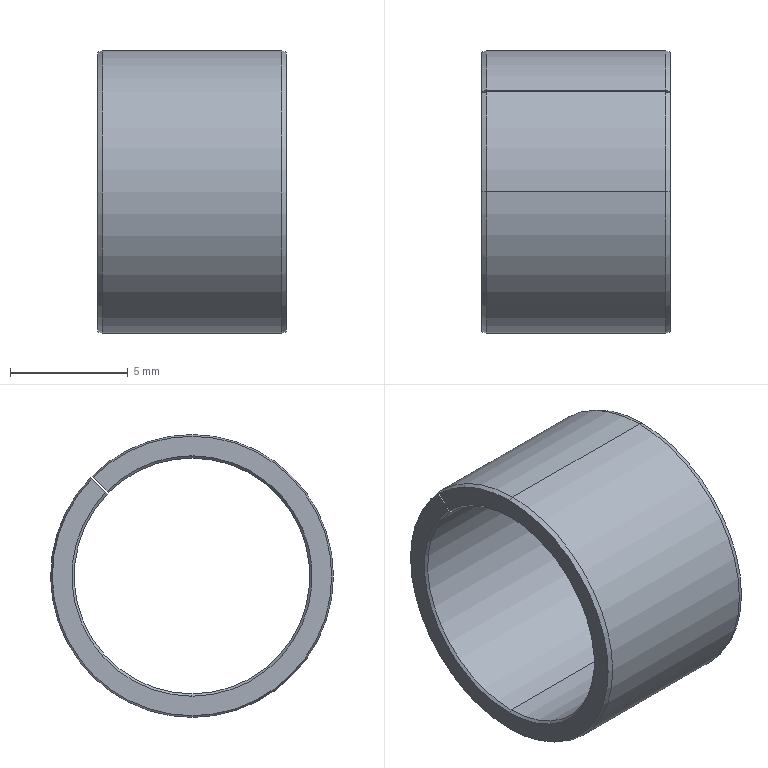Part | STEP file | Flat conveyor mechanism-PCM 101208 E.stp | 1 solid | 22 faces | box 8 x 12 x 12 mm | volume 274.832 mm3 | cone 12 | cylinder 6 | plane 4 | commonest cylinder face diameters 10 x3 12 x3
STEP:
#1=CARTESIAN_POINT('',(0.1,0.,5.));
#2=VERTEX_POINT('',#1);
#3=CARTESIAN_POINT('',(0.1,0.,-5.));
#4=VERTEX_POINT('',#3);
#5=CARTESIAN_POINT('',(0.1,0.,0.));
#6=DIRECTION('',(1.,0.,0.));
#7=DIRECTION('',(0.,0.,-1.));
#8=AXIS2_PLACEMENT_3D('',#5,#6,#7);
#9=CIRCLE('',#8,5.);
#10=EDGE_CURVE('',#2,#4,#9,.T.);
#11=ORIENTED_EDGE('',*,*,#10,.T.);
#12=CARTESIAN_POINT('',(0.,0.,-5.1));
#13=VERTEX_POINT('',#12);
#14=CARTESIAN_POINT('',(0.,0.,-5.1));
#15=DIRECTION('',(-0.7071,0.,-0.7071));
#16=VECTOR('',#15,1000.);
#17=LINE('',#14,#16);
#18=EDGE_CURVE('',#4,#13,#17,.T.);
#19=ORIENTED_EDGE('',*,*,#18,.T.);
#20=CARTESIAN_POINT('',(0.,0.,5.1));
#21=VERTEX_POINT('',#20);
#22=CARTESIAN_POINT('',(0.,0.,0.));
#23=DIRECTION('',(1.,0.,0.));
#24=DIRECTION('',(0.,0.,-1.));
#25=AXIS2_PLACEMENT_3D('',#22,#23,#24);
#26=CIRCLE('',#25,5.1);
#27=EDGE_CURVE('',#21,#13,#26,.T.);
#28=ORIENTED_EDGE('',*,*,#27,.F.);
#29=CARTESIAN_POINT('',(0.,0.,5.1));
#30=DIRECTION('',(-0.7071,0.,0.7071));
#31=VECTOR('',#30,1000.);
#32=LINE('',#29,#31);
#33=EDGE_CURVE('',#2,#21,#32,.T.);
#34=ORIENTED_EDGE('',*,*,#33,.F.);
#35=EDGE_LOOP('',(#11,#19,#28,#34));
#36=FACE_OUTER_BOUND('',#35,.T.);
#37=CARTESIAN_POINT('',(0.,0.,0.));
#38=DIRECTION('',(-1.,0.,0.));
#39=DIRECTION('',(0.,0.,1.));
#40=AXIS2_PLACEMENT_3D('',#37,#38,#39);
#41=CONICAL_SURFACE('',#40,5.1,0.7854);
#42=ADVANCED_FACE('',(#36),#41,.F.);
#43=CARTESIAN_POINT('',(0.1,3.536,3.536));
#44=VERTEX_POINT('',#43);
#45=CARTESIAN_POINT('',(0.1,0.,0.));
#46=DIRECTION('',(1.,0.,0.));
#47=DIRECTION('',(0.,0.,-1.));
#48=AXIS2_PLACEMENT_3D('',#45,#46,#47);
#49=CIRCLE('',#48,5.);
#50=EDGE_CURVE('',#44,#2,#49,.T.);
#51=ORIENTED_EDGE('',*,*,#50,.T.);
#52=ORIENTED_EDGE('',*,*,#33,.T.);
#53=CARTESIAN_POINT('',(0.,3.606,3.606));
#54=VERTEX_POINT('',#53);
#55=CARTESIAN_POINT('',(0.,0.,0.));
#56=DIRECTION('',(1.,0.,0.));
#57=DIRECTION('',(0.,0.,-1.));
#58=AXIS2_PLACEMENT_3D('',#55,#56,#57);
#59=CIRCLE('',#58,5.1);
#60=EDGE_CURVE('',#54,#21,#59,.T.);
#61=ORIENTED_EDGE('',*,*,#60,.F.);
#62=CARTESIAN_POINT('',(0.,3.606,3.606));
#63=DIRECTION('',(0.7071,-0.5,-0.5));
#64=VECTOR('',#63,1000.);
#65=LINE('',#62,#64);
#66=EDGE_CURVE('',#54,#44,#65,.T.);
#67=ORIENTED_EDGE('',*,*,#66,.T.);
#68=EDGE_LOOP('',(#51,#52,#61,#67));
#69=FACE_OUTER_BOUND('',#68,.T.);
#70=CARTESIAN_POINT('',(0.,0.,0.));
#71=DIRECTION('',(-1.,0.,0.));
#72=DIRECTION('',(0.,0.,1.));
#73=AXIS2_PLACEMENT_3D('',#70,#71,#72);
#74=CONICAL_SURFACE('',#73,5.1,0.7854);
#75=ADVANCED_FACE('',(#69),#74,.F.);
#76=CARTESIAN_POINT('',(7.9,3.536,3.536));
#77=VERTEX_POINT('',#76);
#78=CARTESIAN_POINT('',(7.9,0.,5.));
#79=VERTEX_POINT('',#78);
#80=CARTESIAN_POINT('',(7.9,0.,0.));
#81=DIRECTION('',(1.,0.,0.));
#82=DIRECTION('',(0.,0.,-1.));
#83=AXIS2_PLACEMENT_3D('',#80,#81,#82);
#84=CIRCLE('',#83,5.);
#85=EDGE_CURVE('',#77,#79,#84,.T.);
#86=ORIENTED_EDGE('',*,*,#85,.T.);
#87=CARTESIAN_POINT('',(8.,0.,5.));
#88=DIRECTION('',(-1.,0.,0.));
#89=VECTOR('',#88,1000.);
#90=LINE('',#87,#89);
#91=EDGE_CURVE('',#79,#2,#90,.T.);
#92=ORIENTED_EDGE('',*,*,#91,.T.);
#93=ORIENTED_EDGE('',*,*,#50,.F.);
#94=CARTESIAN_POINT('',(0.1,3.536,3.536));
#95=DIRECTION('',(1.,0.,0.));
#96=VECTOR('',#95,1000.);
#97=LINE('',#94,#96);
#98=EDGE_CURVE('',#44,#77,#97,.T.);
#99=ORIENTED_EDGE('',*,*,#98,.T.);
#100=EDGE_LOOP('',(#86,#92,#93,#99));
#101=FACE_OUTER_BOUND('',#100,.T.);
#102=CARTESIAN_POINT('',(8.,0.,0.));
#103=DIRECTION('',(-1.,0.,0.));
#104=DIRECTION('',(0.,0.,-1.));
#105=AXIS2_PLACEMENT_3D('',#102,#103,#104);
#106=CYLINDRICAL_SURFACE('',#105,5.);
#107=ADVANCED_FACE('',(#101),#106,.F.);
#108=ORIENTED_EDGE('',*,*,#91,.F.);
#109=CARTESIAN_POINT('',(7.9,0.,-5.));
#110=VERTEX_POINT('',#109);
#111=CARTESIAN_POINT('',(7.9,0.,0.));
#112=DIRECTION('',(1.,0.,0.));
#113=DIRECTION('',(0.,0.,-1.));
#114=AXIS2_PLACEMENT_3D('',#111,#112,#113);
#115=CIRCLE('',#114,5.);
#116=EDGE_CURVE('',#79,#110,#115,.T.);
#117=ORIENTED_EDGE('',*,*,#116,.T.);
#118=CARTESIAN_POINT('',(8.,0.,-5.));
#119=DIRECTION('',(-1.,0.,0.));
#120=VECTOR('',#119,1000.);
#121=LINE('',#118,#120);
#122=EDGE_CURVE('',#110,#4,#121,.T.);
#123=ORIENTED_EDGE('',*,*,#122,.T.);
#124=ORIENTED_EDGE('',*,*,#10,.F.);
#125=EDGE_LOOP('',(#108,#117,#123,#124));
#126=FACE_OUTER_BOUND('',#125,.T.);
#127=CARTESIAN_POINT('',(8.,0.,0.));
#128=DIRECTION('',(-1.,0.,0.));
#129=DIRECTION('',(0.,0.,-1.));
#130=AXIS2_PLACEMENT_3D('',#127,#128,#129);
#131=CYLINDRICAL_SURFACE('',#130,5.);
#132=ADVANCED_FACE('',(#126),#131,.F.);
#133=ORIENTED_EDGE('',*,*,#116,.F.);
#134=CARTESIAN_POINT('',(8.,0.,5.1));
#135=VERTEX_POINT('',#134);
#136=CARTESIAN_POINT('',(7.9,0.,5.));
#137=DIRECTION('',(0.7071,0.,0.7071));
#138=VECTOR('',#137,1000.);
#139=LINE('',#136,#138);
#140=EDGE_CURVE('',#79,#135,#139,.T.);
#141=ORIENTED_EDGE('',*,*,#140,.T.);
#142=CARTESIAN_POINT('',(8.,0.,-5.1));
#143=VERTEX_POINT('',#142);
#144=CARTESIAN_POINT('',(8.,0.,0.));
#145=DIRECTION('',(1.,0.,0.));
#146=DIRECTION('',(0.,0.,-1.));
#147=AXIS2_PLACEMENT_3D('',#144,#145,#146);
#148=CIRCLE('',#147,5.1);
#149=EDGE_CURVE('',#135,#143,#148,.T.);
#150=ORIENTED_EDGE('',*,*,#149,.T.);
#151=CARTESIAN_POINT('',(7.9,0.,-5.));
#152=DIRECTION('',(0.7071,0.,-0.7071));
#153=VECTOR('',#152,1000.);
#154=LINE('',#151,#153);
#155=EDGE_CURVE('',#110,#143,#154,.T.);
#156=ORIENTED_EDGE('',*,*,#155,.F.);
#157=EDGE_LOOP('',(#133,#141,#150,#156));
#158=FACE_OUTER_BOUND('',#157,.T.);
#159=CARTESIAN_POINT('',(7.9,0.,0.));
#160=DIRECTION('',(1.,0.,0.));
#161=DIRECTION('',(0.,0.,-1.));
#162=AXIS2_PLACEMENT_3D('',#159,#160,#161);
#163=CONICAL_SURFACE('',#162,5.,0.7854);
#164=ADVANCED_FACE('',(#158),#163,.F.);
#165=CARTESIAN_POINT('',(7.9,3.597,3.473));
#166=VERTEX_POINT('',#165);
#167=CARTESIAN_POINT('',(7.9,0.,0.));
#168=DIRECTION('',(1.,0.,0.));
#169=DIRECTION('',(0.,0.,-1.));
#170=AXIS2_PLACEMENT_3D('',#167,#168,#169);
#171=CIRCLE('',#170,5.);
#172=EDGE_CURVE('',#110,#166,#171,.T.);
#173=ORIENTED_EDGE('',*,*,#172,.F.);
#174=ORIENTED_EDGE('',*,*,#155,.T.);
#175=CARTESIAN_POINT('',(8.,3.669,3.543));
#176=VERTEX_POINT('',#175);
#177=CARTESIAN_POINT('',(8.,0.,0.));
#178=DIRECTION('',(1.,0.,0.));
#179=DIRECTION('',(0.,0.,-1.));
#180=AXIS2_PLACEMENT_3D('',#177,#178,#179);
#181=CIRCLE('',#180,5.1);
#182=EDGE_CURVE('',#143,#176,#181,.T.);
#183=ORIENTED_EDGE('',*,*,#182,.T.);
#184=CARTESIAN_POINT('',(7.9,3.597,3.473));
#185=DIRECTION('',(0.7071,0.5087,0.4912));
#186=VECTOR('',#185,1000.);
#187=LINE('',#184,#186);
#188=EDGE_CURVE('',#166,#176,#187,.T.);
#189=ORIENTED_EDGE('',*,*,#188,.F.);
#190=EDGE_LOOP('',(#173,#174,#183,#189));
#191=FACE_OUTER_BOUND('',#190,.T.);
#192=CARTESIAN_POINT('',(7.9,0.,0.));
#193=DIRECTION('',(1.,0.,0.));
#194=DIRECTION('',(0.,0.,-1.));
#195=AXIS2_PLACEMENT_3D('',#192,#193,#194);
#196=CONICAL_SURFACE('',#195,5.,0.7854);
#197=ADVANCED_FACE('',(#191),#196,.F.);
#198=CARTESIAN_POINT('',(8.,0.,-5.927));
#199=VERTEX_POINT('',#198);
#200=CARTESIAN_POINT('',(8.,4.264,4.117));
#201=VERTEX_POINT('',#200);
#202=CARTESIAN_POINT('',(8.,0.,0.));
#203=DIRECTION('',(1.,0.,0.));
#204=DIRECTION('',(0.,0.,-1.));
#205=AXIS2_PLACEMENT_3D('',#202,#203,#204);
#206=CIRCLE('',#205,5.927);
#207=EDGE_CURVE('',#199,#201,#206,.T.);
#208=ORIENTED_EDGE('',*,*,#207,.F.);
#209=CARTESIAN_POINT('',(7.8,0.,-6.));
#210=VERTEX_POINT('',#209);
#211=CARTESIAN_POINT('',(8.,0.,-5.927));
#212=DIRECTION('',(-0.9397,0.,-0.342));
#213=VECTOR('',#212,1000.);
#214=LINE('',#211,#213);
#215=EDGE_CURVE('',#199,#210,#214,.T.);
#216=ORIENTED_EDGE('',*,*,#215,.T.);
#217=CARTESIAN_POINT('',(7.8,4.316,4.168));
#218=VERTEX_POINT('',#217);
#219=CARTESIAN_POINT('',(7.8,0.,0.));
#220=DIRECTION('',(1.,0.,0.));
#221=DIRECTION('',(0.,0.,-1.));
#222=AXIS2_PLACEMENT_3D('',#219,#220,#221);
#223=CIRCLE('',#222,6.);
#224=EDGE_CURVE('',#210,#218,#223,.T.);
#225=ORIENTED_EDGE('',*,*,#224,.T.);
#226=CARTESIAN_POINT('',(8.,4.264,4.117));
#227=DIRECTION('',(-0.9397,0.246,0.2376));
#228=VECTOR('',#227,1000.);
#229=LINE('',#226,#228);
#230=EDGE_CURVE('',#201,#218,#229,.T.);
#231=ORIENTED_EDGE('',*,*,#230,.F.);
#232=EDGE_LOOP('',(#208,#216,#225,#231));
#233=FACE_OUTER_BOUND('',#232,.T.);
#234=CARTESIAN_POINT('',(8.,0.,0.));
#235=DIRECTION('',(-1.,0.,0.));
#236=DIRECTION('',(0.,0.,1.));
#237=AXIS2_PLACEMENT_3D('',#234,#235,#236);
#238=CONICAL_SURFACE('',#237,5.927,0.3491);
#239=ADVANCED_FACE('',(#233),#238,.T.);
#240=ORIENTED_EDGE('',*,*,#215,.F.);
#241=CARTESIAN_POINT('',(8.,0.,5.927));
#242=VERTEX_POINT('',#241);
#243=CARTESIAN_POINT('',(8.,0.,0.));
#244=DIRECTION('',(1.,0.,0.));
#245=DIRECTION('',(0.,0.,-1.));
#246=AXIS2_PLACEMENT_3D('',#243,#244,#245);
#247=CIRCLE('',#246,5.927);
#248=EDGE_CURVE('',#242,#199,#247,.T.);
#249=ORIENTED_EDGE('',*,*,#248,.F.);
#250=CARTESIAN_POINT('',(7.8,0.,6.));
#251=VERTEX_POINT('',#250);
#252=CARTESIAN_POINT('',(8.,0.,5.927));
#253=DIRECTION('',(-0.9397,0.,0.342));
#254=VECTOR('',#253,1000.);
#255=LINE('',#252,#254);
#256=EDGE_CURVE('',#242,#251,#255,.T.);
#257=ORIENTED_EDGE('',*,*,#256,.T.);
#258=CARTESIAN_POINT('',(7.8,0.,0.));
#259=DIRECTION('',(1.,0.,0.));
#260=DIRECTION('',(0.,0.,-1.));
#261=AXIS2_PLACEMENT_3D('',#258,#259,#260);
#262=CIRCLE('',#261,6.);
#263=EDGE_CURVE('',#251,#210,#262,.T.);
#264=ORIENTED_EDGE('',*,*,#263,.T.);
#265=EDGE_LOOP('',(#240,#249,#257,#264));
#266=FACE_OUTER_BOUND('',#265,.T.);
#267=CARTESIAN_POINT('',(8.,0.,0.));
#268=DIRECTION('',(-1.,0.,0.));
#269=DIRECTION('',(0.,0.,1.));
#270=AXIS2_PLACEMENT_3D('',#267,#268,#269);
#271=CONICAL_SURFACE('',#270,5.927,0.3491);
#272=ADVANCED_FACE('',(#266),#271,.T.);
#273=CARTESIAN_POINT('',(0.,4.191,4.191));
#274=VERTEX_POINT('',#273);
#275=CARTESIAN_POINT('',(0.,0.,5.927));
#276=VERTEX_POINT('',#275);
#277=CARTESIAN_POINT('',(0.,0.,0.));
#278=DIRECTION('',(1.,0.,0.));
#279=DIRECTION('',(0.,0.,-1.));
#280=AXIS2_PLACEMENT_3D('',#277,#278,#279);
#281=CIRCLE('',#280,5.927);
#282=EDGE_CURVE('',#274,#276,#281,.T.);
#283=ORIENTED_EDGE('',*,*,#282,.T.);
#284=CARTESIAN_POINT('',(0.2,0.,6.));
#285=VERTEX_POINT('',#284);
#286=CARTESIAN_POINT('',(0.2,0.,6.));
#287=DIRECTION('',(0.9397,0.,0.342));
#288=VECTOR('',#287,1000.);
#289=LINE('',#286,#288);
#290=EDGE_CURVE('',#276,#285,#289,.T.);
#291=ORIENTED_EDGE('',*,*,#290,.T.);
#292=CARTESIAN_POINT('',(0.2,4.243,4.243));
#293=VERTEX_POINT('',#292);
#294=CARTESIAN_POINT('',(0.2,0.,0.));
#295=DIRECTION('',(1.,0.,0.));
#296=DIRECTION('',(0.,0.,-1.));
#297=AXIS2_PLACEMENT_3D('',#294,#295,#296);
#298=CIRCLE('',#297,6.);
#299=EDGE_CURVE('',#293,#285,#298,.T.);
#300=ORIENTED_EDGE('',*,*,#299,.F.);
#301=CARTESIAN_POINT('',(0.2,4.243,4.243));
#302=DIRECTION('',(-0.9397,-0.2418,-0.2418));
#303=VECTOR('',#302,1000.);
#304=LINE('',#301,#303);
#305=EDGE_CURVE('',#293,#274,#304,.T.);
#306=ORIENTED_EDGE('',*,*,#305,.T.);
#307=EDGE_LOOP('',(#283,#291,#300,#306));
#308=FACE_OUTER_BOUND('',#307,.T.);
#309=CARTESIAN_POINT('',(0.2,0.,0.));
#310=DIRECTION('',(1.,0.,0.));
#311=DIRECTION('',(0.,0.,-1.));
#312=AXIS2_PLACEMENT_3D('',#309,#310,#311);
#313=CONICAL_SURFACE('',#312,6.,0.3491);
#314=ADVANCED_FACE('',(#308),#313,.T.);
#315=ORIENTED_EDGE('',*,*,#290,.F.);
#316=CARTESIAN_POINT('',(0.,0.,-5.927));
#317=VERTEX_POINT('',#316);
#318=CARTESIAN_POINT('',(0.,0.,0.));
#319=DIRECTION('',(1.,0.,0.));
#320=DIRECTION('',(0.,0.,-1.));
#321=AXIS2_PLACEMENT_3D('',#318,#319,#320);
#322=CIRCLE('',#321,5.927);
#323=EDGE_CURVE('',#276,#317,#322,.T.);
#324=ORIENTED_EDGE('',*,*,#323,.T.);
#325=CARTESIAN_POINT('',(0.2,0.,-6.));
#326=VERTEX_POINT('',#325);
#327=CARTESIAN_POINT('',(0.2,0.,-6.));
#328=DIRECTION('',(0.9397,0.,-0.342));
#329=VECTOR('',#328,1000.);
#330=LINE('',#327,#329);
#331=EDGE_CURVE('',#317,#326,#330,.T.);
#332=ORIENTED_EDGE('',*,*,#331,.T.);
#333=CARTESIAN_POINT('',(0.2,0.,0.));
#334=DIRECTION('',(1.,0.,0.));
#335=DIRECTION('',(0.,0.,-1.));
#336=AXIS2_PLACEMENT_3D('',#333,#334,#335);
#337=CIRCLE('',#336,6.);
#338=EDGE_CURVE('',#285,#326,#337,.T.);
#339=ORIENTED_EDGE('',*,*,#338,.F.);
#340=EDGE_LOOP('',(#315,#324,#332,#339));
#341=FACE_OUTER_BOUND('',#340,.T.);
#342=CARTESIAN_POINT('',(0.2,0.,0.));
#343=DIRECTION('',(1.,0.,0.));
#344=DIRECTION('',(0.,0.,-1.));
#345=AXIS2_PLACEMENT_3D('',#342,#343,#344);
#346=CONICAL_SURFACE('',#345,6.,0.3491);
#347=ADVANCED_FACE('',(#341),#346,.T.);
#348=ORIENTED_EDGE('',*,*,#263,.F.);
#349=CARTESIAN_POINT('',(8.,0.,6.));
#350=DIRECTION('',(-1.,0.,0.));
#351=VECTOR('',#350,1000.);
#352=LINE('',#349,#351);
#353=EDGE_CURVE('',#251,#285,#352,.T.);
#354=ORIENTED_EDGE('',*,*,#353,.T.);
#355=ORIENTED_EDGE('',*,*,#338,.T.);
#356=CARTESIAN_POINT('',(8.,0.,-6.));
#357=DIRECTION('',(-1.,0.,0.));
#358=VECTOR('',#357,1000.);
#359=LINE('',#356,#358);
#360=EDGE_CURVE('',#210,#326,#359,.T.);
#361=ORIENTED_EDGE('',*,*,#360,.F.);
#362=EDGE_LOOP('',(#348,#354,#355,#361));
#363=FACE_OUTER_BOUND('',#362,.T.);
#364=CARTESIAN_POINT('',(8.,0.,0.));
#365=DIRECTION('',(-1.,0.,0.));
#366=DIRECTION('',(0.,0.,-1.));
#367=AXIS2_PLACEMENT_3D('',#364,#365,#366);
#368=CYLINDRICAL_SURFACE('',#367,6.);
#369=ADVANCED_FACE('',(#363),#368,.T.);
#370=ORIENTED_EDGE('',*,*,#224,.F.);
#371=ORIENTED_EDGE('',*,*,#360,.T.);
#372=CARTESIAN_POINT('',(0.2,4.316,4.168));
#373=VERTEX_POINT('',#372);
#374=CARTESIAN_POINT('',(0.2,0.,0.));
#375=DIRECTION('',(1.,0.,0.));
#376=DIRECTION('',(0.,0.,-1.));
#377=AXIS2_PLACEMENT_3D('',#374,#375,#376);
#378=CIRCLE('',#377,6.);
#379=EDGE_CURVE('',#326,#373,#378,.T.);
#380=ORIENTED_EDGE('',*,*,#379,.T.);
#381=CARTESIAN_POINT('',(7.8,4.316,4.168));
#382=DIRECTION('',(-1.,0.,0.));
#383=VECTOR('',#382,1000.);
#384=LINE('',#381,#383);
#385=EDGE_CURVE('',#218,#373,#384,.T.);
#386=ORIENTED_EDGE('',*,*,#385,.F.);
#387=EDGE_LOOP('',(#370,#371,#380,#386));
#388=FACE_OUTER_BOUND('',#387,.T.);
#389=CARTESIAN_POINT('',(8.,0.,0.));
#390=DIRECTION('',(-1.,0.,0.));
#391=DIRECTION('',(0.,0.,-1.));
#392=AXIS2_PLACEMENT_3D('',#389,#390,#391);
#393=CYLINDRICAL_SURFACE('',#392,6.);
#394=ADVANCED_FACE('',(#388),#393,.T.);
#395=ORIENTED_EDGE('',*,*,#305,.F.);
#396=CARTESIAN_POINT('',(7.8,4.243,4.243));
#397=VERTEX_POINT('',#396);
#398=CARTESIAN_POINT('',(7.8,4.243,4.243));
#399=DIRECTION('',(-1.,0.,0.));
#400=VECTOR('',#399,1000.);
#401=LINE('',#398,#400);
#402=EDGE_CURVE('',#397,#293,#401,.T.);
#403=ORIENTED_EDGE('',*,*,#402,.F.);
#404=CARTESIAN_POINT('',(8.,4.191,4.191));
#405=VERTEX_POINT('',#404);
#406=CARTESIAN_POINT('',(8.,4.191,4.191));
#407=DIRECTION('',(-0.9397,0.2418,0.2418));
#408=VECTOR('',#407,1000.);
#409=LINE('',#406,#408);
#410=EDGE_CURVE('',#405,#397,#409,.T.);
#411=ORIENTED_EDGE('',*,*,#410,.F.);
#412=CARTESIAN_POINT('',(8.,3.606,3.606));
#413=VERTEX_POINT('',#412);
#414=CARTESIAN_POINT('',(8.,3.606,3.606));
#415=DIRECTION('',(0.,0.7071,0.7071));
#416=VECTOR('',#415,1000.);
#417=LINE('',#414,#416);
#418=EDGE_CURVE('',#413,#405,#417,.T.);
#419=ORIENTED_EDGE('',*,*,#418,.F.);
#420=CARTESIAN_POINT('',(7.9,3.536,3.536));
#421=DIRECTION('',(0.7071,0.5,0.5));
#422=VECTOR('',#421,1000.);
#423=LINE('',#420,#422);
#424=EDGE_CURVE('',#77,#413,#423,.T.);
#425=ORIENTED_EDGE('',*,*,#424,.F.);
#426=ORIENTED_EDGE('',*,*,#98,.F.);
#427=ORIENTED_EDGE('',*,*,#66,.F.);
#428=CARTESIAN_POINT('',(0.,4.191,4.191));
#429=DIRECTION('',(0.,-0.7071,-0.7071));
#430=VECTOR('',#429,1000.);
#431=LINE('',#428,#430);
#432=EDGE_CURVE('',#274,#54,#431,.T.);
#433=ORIENTED_EDGE('',*,*,#432,.F.);
#434=EDGE_LOOP('',(#395,#403,#411,#419,#425,#426,#427,#433));
#435=FACE_OUTER_BOUND('',#434,.T.);
#436=CARTESIAN_POINT('',(0.,0.,0.));
#437=DIRECTION('',(0.,-0.7071,0.7071));
#438=DIRECTION('',(-1.,0.,0.));
#439=AXIS2_PLACEMENT_3D('',#436,#437,#438);
#440=PLANE('',#439);
#441=ADVANCED_FACE('',(#435),#440,.F.);
#442=CARTESIAN_POINT('',(0.,4.264,4.117));
#443=VERTEX_POINT('',#442);
#444=CARTESIAN_POINT('',(0.2,4.316,4.168));
#445=DIRECTION('',(-0.9397,-0.246,-0.2376));
#446=VECTOR('',#445,1000.);
#447=LINE('',#444,#446);
#448=EDGE_CURVE('',#373,#443,#447,.T.);
#449=ORIENTED_EDGE('',*,*,#448,.T.);
#450=CARTESIAN_POINT('',(0.,3.669,3.543));
#451=VERTEX_POINT('',#450);
#452=CARTESIAN_POINT('',(0.,4.264,4.117));
#453=DIRECTION('',(0.,-0.7193,-0.6947));
#454=VECTOR('',#453,1000.);
#455=LINE('',#452,#454);
#456=EDGE_CURVE('',#443,#451,#455,.T.);
#457=ORIENTED_EDGE('',*,*,#456,.T.);
#458=CARTESIAN_POINT('',(0.1,3.597,3.473));
#459=VERTEX_POINT('',#458);
#460=CARTESIAN_POINT('',(0.,3.669,3.543));
#461=DIRECTION('',(0.7071,-0.5087,-0.4912));
#462=VECTOR('',#461,1000.);
#463=LINE('',#460,#462);
#464=EDGE_CURVE('',#451,#459,#463,.T.);
#465=ORIENTED_EDGE('',*,*,#464,.T.);
#466=CARTESIAN_POINT('',(0.1,3.597,3.473));
#467=DIRECTION('',(1.,0.,0.));
#468=VECTOR('',#467,1000.);
#469=LINE('',#466,#468);
#470=EDGE_CURVE('',#459,#166,#469,.T.);
#471=ORIENTED_EDGE('',*,*,#470,.T.);
#472=ORIENTED_EDGE('',*,*,#188,.T.);
#473=CARTESIAN_POINT('',(8.,3.669,3.543));
#474=DIRECTION('',(0.,0.7193,0.6947));
#475=VECTOR('',#474,1000.);
#476=LINE('',#473,#475);
#477=EDGE_CURVE('',#176,#201,#476,.T.);
#478=ORIENTED_EDGE('',*,*,#477,.T.);
#479=ORIENTED_EDGE('',*,*,#230,.T.);
#480=ORIENTED_EDGE('',*,*,#385,.T.);
#481=EDGE_LOOP('',(#449,#457,#465,#471,#472,#478,#479,#480));
#482=FACE_OUTER_BOUND('',#481,.T.);
#483=CARTESIAN_POINT('',(0.,0.,0.));
#484=DIRECTION('',(0.,-0.6947,0.7193));
#485=DIRECTION('',(-1.,0.,0.));
#486=AXIS2_PLACEMENT_3D('',#483,#484,#485);
#487=PLANE('',#486);
#488=ADVANCED_FACE('',(#482),#487,.T.);
#489=ORIENTED_EDGE('',*,*,#353,.F.);
#490=CARTESIAN_POINT('',(7.8,0.,0.));
#491=DIRECTION('',(1.,0.,0.));
#492=DIRECTION('',(0.,0.,-1.));
#493=AXIS2_PLACEMENT_3D('',#490,#491,#492);
#494=CIRCLE('',#493,6.);
#495=EDGE_CURVE('',#397,#251,#494,.T.);
#496=ORIENTED_EDGE('',*,*,#495,.F.);
#497=ORIENTED_EDGE('',*,*,#402,.T.);
#498=ORIENTED_EDGE('',*,*,#299,.T.);
#499=EDGE_LOOP('',(#489,#496,#497,#498));
#500=FACE_OUTER_BOUND('',#499,.T.);
#501=CARTESIAN_POINT('',(8.,0.,0.));
#502=DIRECTION('',(-1.,0.,0.));
#503=DIRECTION('',(0.,0.,-1.));
#504=AXIS2_PLACEMENT_3D('',#501,#502,#503);
#505=CYLINDRICAL_SURFACE('',#504,6.);
#506=ADVANCED_FACE('',(#500),#505,.T.);
#507=ORIENTED_EDGE('',*,*,#331,.F.);
#508=CARTESIAN_POINT('',(0.,0.,0.));
#509=DIRECTION('',(1.,0.,0.));
#510=DIRECTION('',(0.,0.,-1.));
#511=AXIS2_PLACEMENT_3D('',#508,#509,#510);
#512=CIRCLE('',#511,5.927);
#513=EDGE_CURVE('',#317,#443,#512,.T.);
#514=ORIENTED_EDGE('',*,*,#513,.T.);
#515=ORIENTED_EDGE('',*,*,#448,.F.);
#516=ORIENTED_EDGE('',*,*,#379,.F.);
#517=EDGE_LOOP('',(#507,#514,#515,#516));
#518=FACE_OUTER_BOUND('',#517,.T.);
#519=CARTESIAN_POINT('',(0.2,0.,0.));
#520=DIRECTION('',(1.,0.,0.));
#521=DIRECTION('',(0.,0.,-1.));
#522=AXIS2_PLACEMENT_3D('',#519,#520,#521);
#523=CONICAL_SURFACE('',#522,6.,0.3491);
#524=ADVANCED_FACE('',(#518),#523,.T.);
#525=ORIENTED_EDGE('',*,*,#60,.T.);
#526=ORIENTED_EDGE('',*,*,#27,.T.);
#527=CARTESIAN_POINT('',(0.,0.,0.));
#528=DIRECTION('',(1.,0.,0.));
#529=DIRECTION('',(0.,0.,-1.));
#530=AXIS2_PLACEMENT_3D('',#527,#528,#529);
#531=CIRCLE('',#530,5.1);
#532=EDGE_CURVE('',#13,#451,#531,.T.);
#533=ORIENTED_EDGE('',*,*,#532,.T.);
#534=ORIENTED_EDGE('',*,*,#456,.F.);
#535=ORIENTED_EDGE('',*,*,#513,.F.);
#536=ORIENTED_EDGE('',*,*,#323,.F.);
#537=ORIENTED_EDGE('',*,*,#282,.F.);
#538=ORIENTED_EDGE('',*,*,#432,.T.);
#539=EDGE_LOOP('',(#525,#526,#533,#534,#535,#536,#537,#538));
#540=FACE_OUTER_BOUND('',#539,.T.);
#541=CARTESIAN_POINT('',(0.,4.191,4.191));
#542=DIRECTION('',(-1.,0.,0.));
#543=DIRECTION('',(0.,0.,1.));
#544=AXIS2_PLACEMENT_3D('',#541,#542,#543);
#545=PLANE('',#544);
#546=ADVANCED_FACE('',(#540),#545,.T.);
#547=ORIENTED_EDGE('',*,*,#256,.F.);
#548=CARTESIAN_POINT('',(8.,0.,0.));
#549=DIRECTION('',(1.,0.,0.));
#550=DIRECTION('',(0.,0.,-1.));
#551=AXIS2_PLACEMENT_3D('',#548,#549,#550);
#552=CIRCLE('',#551,5.927);
#553=EDGE_CURVE('',#405,#242,#552,.T.);
#554=ORIENTED_EDGE('',*,*,#553,.F.);
#555=ORIENTED_EDGE('',*,*,#410,.T.);
#556=ORIENTED_EDGE('',*,*,#495,.T.);
#557=EDGE_LOOP('',(#547,#554,#555,#556));
#558=FACE_OUTER_BOUND('',#557,.T.);
#559=CARTESIAN_POINT('',(8.,0.,0.));
#560=DIRECTION('',(-1.,0.,0.));
#561=DIRECTION('',(0.,0.,1.));
#562=AXIS2_PLACEMENT_3D('',#559,#560,#561);
#563=CONICAL_SURFACE('',#562,5.927,0.3491);
#564=ADVANCED_FACE('',(#558),#563,.T.);
#565=ORIENTED_EDGE('',*,*,#553,.T.);
#566=ORIENTED_EDGE('',*,*,#248,.T.);
#567=ORIENTED_EDGE('',*,*,#207,.T.);
#568=ORIENTED_EDGE('',*,*,#477,.F.);
#569=ORIENTED_EDGE('',*,*,#182,.F.);
#570=ORIENTED_EDGE('',*,*,#149,.F.);
#571=CARTESIAN_POINT('',(8.,0.,0.));
#572=DIRECTION('',(1.,0.,0.));
#573=DIRECTION('',(0.,0.,-1.));
#574=AXIS2_PLACEMENT_3D('',#571,#572,#573);
#575=CIRCLE('',#574,5.1);
#576=EDGE_CURVE('',#413,#135,#575,.T.);
#577=ORIENTED_EDGE('',*,*,#576,.F.);
#578=ORIENTED_EDGE('',*,*,#418,.T.);
#579=EDGE_LOOP('',(#565,#566,#567,#568,#569,#570,#577,#578));
#580=FACE_OUTER_BOUND('',#579,.T.);
#581=CARTESIAN_POINT('',(8.,3.606,3.606));
#582=DIRECTION('',(1.,0.,0.));
#583=DIRECTION('',(0.,1.,0.));
#584=AXIS2_PLACEMENT_3D('',#581,#582,#583);
#585=PLANE('',#584);
#586=ADVANCED_FACE('',(#580),#585,.T.);
#587=ORIENTED_EDGE('',*,*,#140,.F.);
#588=ORIENTED_EDGE('',*,*,#85,.F.);
#589=ORIENTED_EDGE('',*,*,#424,.T.);
#590=ORIENTED_EDGE('',*,*,#576,.T.);
#591=EDGE_LOOP('',(#587,#588,#589,#590));
#592=FACE_OUTER_BOUND('',#591,.T.);
#593=CARTESIAN_POINT('',(7.9,0.,0.));
#594=DIRECTION('',(1.,0.,0.));
#595=DIRECTION('',(0.,0.,-1.));
#596=AXIS2_PLACEMENT_3D('',#593,#594,#595);
#597=CONICAL_SURFACE('',#596,5.,0.7854);
#598=ADVANCED_FACE('',(#592),#597,.F.);
#599=ORIENTED_EDGE('',*,*,#122,.F.);
#600=ORIENTED_EDGE('',*,*,#172,.T.);
#601=ORIENTED_EDGE('',*,*,#470,.F.);
#602=CARTESIAN_POINT('',(0.1,0.,0.));
#603=DIRECTION('',(1.,0.,0.));
#604=DIRECTION('',(0.,0.,-1.));
#605=AXIS2_PLACEMENT_3D('',#602,#603,#604);
#606=CIRCLE('',#605,5.);
#607=EDGE_CURVE('',#4,#459,#606,.T.);
#608=ORIENTED_EDGE('',*,*,#607,.F.);
#609=EDGE_LOOP('',(#599,#600,#601,#608));
#610=FACE_OUTER_BOUND('',#609,.T.);
#611=CARTESIAN_POINT('',(8.,0.,0.));
#612=DIRECTION('',(-1.,0.,0.));
#613=DIRECTION('',(0.,0.,-1.));
#614=AXIS2_PLACEMENT_3D('',#611,#612,#613);
#615=CYLINDRICAL_SURFACE('',#614,5.);
#616=ADVANCED_FACE('',(#610),#615,.F.);
#617=ORIENTED_EDGE('',*,*,#18,.F.);
#618=ORIENTED_EDGE('',*,*,#607,.T.);
#619=ORIENTED_EDGE('',*,*,#464,.F.);
#620=ORIENTED_EDGE('',*,*,#532,.F.);
#621=EDGE_LOOP('',(#617,#618,#619,#620));
#622=FACE_OUTER_BOUND('',#621,.T.);
#623=CARTESIAN_POINT('',(0.,0.,0.));
#624=DIRECTION('',(-1.,0.,0.));
#625=DIRECTION('',(0.,0.,1.));
#626=AXIS2_PLACEMENT_3D('',#623,#624,#625);
#627=CONICAL_SURFACE('',#626,5.1,0.7854);
#628=ADVANCED_FACE('',(#622),#627,.F.);
#629=CLOSED_SHELL('',(#42,#75,#107,#132,#164,#197,#239,#272,#314,#347,#369,#394,#441,#488,#506,#524,#546,#564,#586,#598,#616,#628));
#630=MANIFOLD_SOLID_BREP('',#629);
#631=CARTESIAN_POINT('',(0.,0.,0.));
#632=DIRECTION('',(0.,0.,1.));
#633=DIRECTION('',(1.,0.,0.));
#634=AXIS2_PLACEMENT_3D('',#631,#632,#633);
#635=(LENGTH_UNIT()NAMED_UNIT(*)SI_UNIT(.MILLI.,.METRE.));
#636=UNCERTAINTY_MEASURE_WITH_UNIT(LENGTH_MEASURE(0.00001),#635,'','');
#637=(NAMED_UNIT(*)PLANE_ANGLE_UNIT()SI_UNIT($,.RADIAN.));
#638=(NAMED_UNIT(*)SI_UNIT($,.STERADIAN.)SOLID_ANGLE_UNIT());
#639=(GEOMETRIC_REPRESENTATION_CONTEXT(3)GLOBAL_UNCERTAINTY_ASSIGNED_CONTEXT((#636))GLOBAL_UNIT_ASSIGNED_CONTEXT((#635,#637,#638))REPRESENTATION_CONTEXT('',''));
#640=ADVANCED_BREP_SHAPE_REPRESENTATION('',(#630,#634),#639);